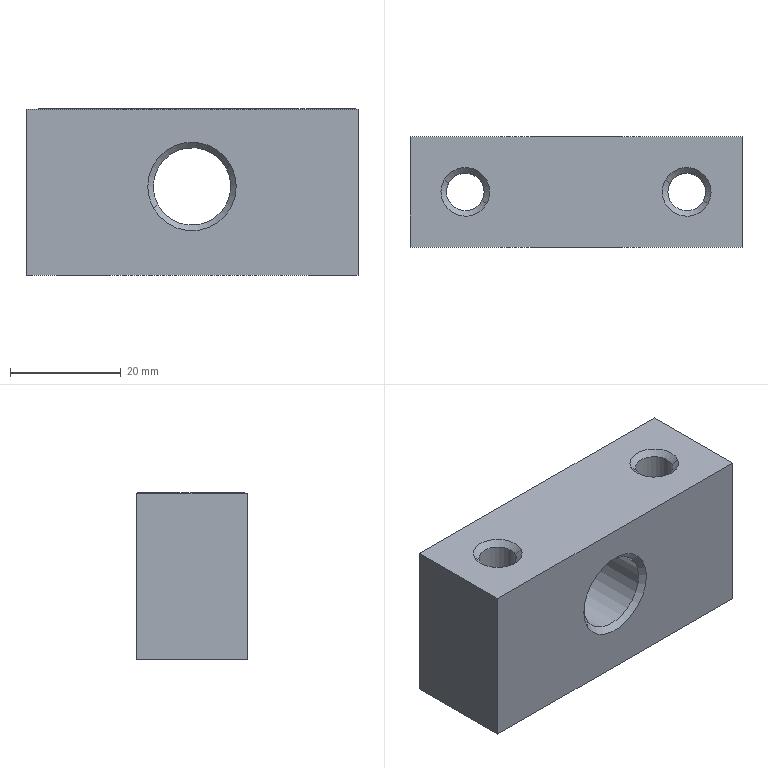Part | STEP file | 20303 | 1 solid | 24 faces | box 60 x 20 x 30 mm | volume 30649 mm3 | cone 12 | plane 6 | cylinder 6 | commonest cylinder face diameters 6.8 x4 14 x2
STEP:
#1=CARTESIAN_POINT('',(30.,-10.,0.));
#2=VERTEX_POINT('',#1);
#3=CARTESIAN_POINT('',(30.,-10.,30.));
#4=VERTEX_POINT('',#3);
#5=CARTESIAN_POINT('',(30.,-10.,15.));
#6=DIRECTION('',(0.,0.,1.));
#7=VECTOR('',#6,1.);
#8=LINE('',#5,#7);
#9=EDGE_CURVE('',#2,#4,#8,.T.);
#10=ORIENTED_EDGE('',*,*,#9,.F.);
#11=CARTESIAN_POINT('',(30.,10.,0.));
#12=VERTEX_POINT('',#11);
#13=CARTESIAN_POINT('',(30.,0.,0.));
#14=DIRECTION('',(0.,-1.,0.));
#15=VECTOR('',#14,1.);
#16=LINE('',#13,#15);
#17=EDGE_CURVE('',#2,#12,#16,.F.);
#18=ORIENTED_EDGE('',*,*,#17,.T.);
#19=CARTESIAN_POINT('',(30.,10.,30.));
#20=VERTEX_POINT('',#19);
#21=CARTESIAN_POINT('',(30.,10.,15.));
#22=DIRECTION('',(0.,0.,1.));
#23=VECTOR('',#22,1.);
#24=LINE('',#21,#23);
#25=EDGE_CURVE('',#12,#20,#24,.T.);
#26=ORIENTED_EDGE('',*,*,#25,.T.);
#27=CARTESIAN_POINT('',(30.,0.,30.));
#28=DIRECTION('',(0.,-1.,0.));
#29=VECTOR('',#28,1.);
#30=LINE('',#27,#29);
#31=EDGE_CURVE('',#4,#20,#30,.F.);
#32=ORIENTED_EDGE('',*,*,#31,.F.);
#33=EDGE_LOOP('',(#10,#18,#26,#32));
#34=FACE_OUTER_BOUND('',#33,.T.);
#35=CARTESIAN_POINT('',(30.,10.,0.));
#36=DIRECTION('',(-1.,0.,0.));
#37=DIRECTION('',(0.,-1.,0.));
#38=AXIS2_PLACEMENT_3D('',#35,#36,#37);
#39=PLANE('',#38);
#40=ADVANCED_FACE('',(#34),#39,.F.);
#41=CARTESIAN_POINT('',(-30.,10.,0.));
#42=VERTEX_POINT('',#41);
#43=CARTESIAN_POINT('',(-30.,10.,30.));
#44=VERTEX_POINT('',#43);
#45=CARTESIAN_POINT('',(-30.,10.,15.));
#46=DIRECTION('',(0.,0.,1.));
#47=VECTOR('',#46,1.);
#48=LINE('',#45,#47);
#49=EDGE_CURVE('',#42,#44,#48,.T.);
#50=ORIENTED_EDGE('',*,*,#49,.F.);
#51=CARTESIAN_POINT('',(-30.,-10.,0.));
#52=VERTEX_POINT('',#51);
#53=CARTESIAN_POINT('',(-30.,0.,0.));
#54=DIRECTION('',(0.,1.,0.));
#55=VECTOR('',#54,1.);
#56=LINE('',#53,#55);
#57=EDGE_CURVE('',#42,#52,#56,.F.);
#58=ORIENTED_EDGE('',*,*,#57,.T.);
#59=CARTESIAN_POINT('',(-30.,-10.,30.));
#60=VERTEX_POINT('',#59);
#61=CARTESIAN_POINT('',(-30.,-10.,15.));
#62=DIRECTION('',(0.,0.,1.));
#63=VECTOR('',#62,1.);
#64=LINE('',#61,#63);
#65=EDGE_CURVE('',#52,#60,#64,.T.);
#66=ORIENTED_EDGE('',*,*,#65,.T.);
#67=CARTESIAN_POINT('',(-30.,0.,30.));
#68=DIRECTION('',(0.,1.,0.));
#69=VECTOR('',#68,1.);
#70=LINE('',#67,#69);
#71=EDGE_CURVE('',#44,#60,#70,.F.);
#72=ORIENTED_EDGE('',*,*,#71,.F.);
#73=EDGE_LOOP('',(#50,#58,#66,#72));
#74=FACE_OUTER_BOUND('',#73,.T.);
#75=CARTESIAN_POINT('',(-30.,-10.,0.));
#76=DIRECTION('',(1.,0.,0.));
#77=DIRECTION('',(0.,1.,0.));
#78=AXIS2_PLACEMENT_3D('',#75,#76,#77);
#79=PLANE('',#78);
#80=ADVANCED_FACE('',(#74),#79,.F.);
#81=CARTESIAN_POINT('',(17.016,1.63,1.));
#82=VERTEX_POINT('',#81);
#83=CARTESIAN_POINT('',(16.139,2.109,0.));
#84=VERTEX_POINT('',#83);
#85=CARTESIAN_POINT('',(16.577,1.87,0.5));
#86=DIRECTION('',(-0.6205,0.339,-0.7071));
#87=VECTOR('',#86,1.);
#88=LINE('',#85,#87);
#89=EDGE_CURVE('',#82,#84,#88,.T.);
#90=ORIENTED_EDGE('',*,*,#89,.T.);
#91=CARTESIAN_POINT('',(23.861,-2.109,0.));
#92=VERTEX_POINT('',#91);
#93=CARTESIAN_POINT('',(20.,0.,0.));
#94=DIRECTION('',(0.,0.,1.));
#95=AXIS2_PLACEMENT_3D('',#93,#94,$);
#96=CIRCLE('',#95,4.4);
#97=EDGE_CURVE('',#84,#92,#96,.F.);
#98=ORIENTED_EDGE('',*,*,#97,.T.);
#99=CARTESIAN_POINT('',(22.984,-1.63,1.));
#100=VERTEX_POINT('',#99);
#101=CARTESIAN_POINT('',(23.423,-1.87,0.5));
#102=DIRECTION('',(0.6205,-0.339,-0.7071));
#103=VECTOR('',#102,1.);
#104=LINE('',#101,#103);
#105=EDGE_CURVE('',#100,#92,#104,.T.);
#106=ORIENTED_EDGE('',*,*,#105,.F.);
#107=CARTESIAN_POINT('',(20.,0.,1.));
#108=DIRECTION('',(0.,0.,1.));
#109=AXIS2_PLACEMENT_3D('',#107,#108,$);
#110=CIRCLE('',#109,3.4);
#111=EDGE_CURVE('',#82,#100,#110,.F.);
#112=ORIENTED_EDGE('',*,*,#111,.F.);
#113=EDGE_LOOP('',(#90,#98,#106,#112));
#114=FACE_OUTER_BOUND('',#113,.T.);
#115=CARTESIAN_POINT('',(20.,0.,4.4));
#116=DIRECTION('',(0.,0.,-1.));
#117=DIRECTION('',(0.8776,-0.4794,0.));
#118=AXIS2_PLACEMENT_3D('',#115,#116,#117);
#119=CONICAL_SURFACE('',#118,0.,0.7854);
#120=ADVANCED_FACE('',(#114),#119,.F.);
#121=ORIENTED_EDGE('',*,*,#105,.T.);
#122=CARTESIAN_POINT('',(20.,0.,0.));
#123=DIRECTION('',(0.,0.,1.));
#124=AXIS2_PLACEMENT_3D('',#122,#123,$);
#125=CIRCLE('',#124,4.4);
#126=EDGE_CURVE('',#92,#84,#125,.F.);
#127=ORIENTED_EDGE('',*,*,#126,.T.);
#128=ORIENTED_EDGE('',*,*,#89,.F.);
#129=CARTESIAN_POINT('',(20.,0.,1.));
#130=DIRECTION('',(0.,0.,1.));
#131=AXIS2_PLACEMENT_3D('',#129,#130,$);
#132=CIRCLE('',#131,3.4);
#133=EDGE_CURVE('',#100,#82,#132,.F.);
#134=ORIENTED_EDGE('',*,*,#133,.F.);
#135=EDGE_LOOP('',(#121,#127,#128,#134));
#136=FACE_OUTER_BOUND('',#135,.T.);
#137=CARTESIAN_POINT('',(20.,0.,4.4));
#138=DIRECTION('',(0.,0.,-1.));
#139=DIRECTION('',(-0.5949,0.8038,0.));
#140=AXIS2_PLACEMENT_3D('',#137,#138,#139);
#141=CONICAL_SURFACE('',#140,0.,0.7854);
#142=ADVANCED_FACE('',(#136),#141,.F.);
#143=CARTESIAN_POINT('',(22.984,-1.63,29.));
#144=VERTEX_POINT('',#143);
#145=CARTESIAN_POINT('',(17.016,1.63,29.));
#146=VERTEX_POINT('',#145);
#147=CARTESIAN_POINT('',(20.,0.,29.));
#148=DIRECTION('',(0.,0.,-1.));
#149=AXIS2_PLACEMENT_3D('',#147,#148,$);
#150=CIRCLE('',#149,3.4);
#151=EDGE_CURVE('',#144,#146,#150,.F.);
#152=ORIENTED_EDGE('',*,*,#151,.T.);
#153=CARTESIAN_POINT('',(17.016,1.63,15.155));
#154=DIRECTION('',(0.,0.,-1.));
#155=VECTOR('',#154,1.);
#156=LINE('',#153,#155);
#157=EDGE_CURVE('',#82,#146,#156,.F.);
#158=ORIENTED_EDGE('',*,*,#157,.F.);
#159=ORIENTED_EDGE('',*,*,#111,.T.);
#160=CARTESIAN_POINT('',(22.984,-1.63,15.155));
#161=DIRECTION('',(0.,0.,-1.));
#162=VECTOR('',#161,1.);
#163=LINE('',#160,#162);
#164=EDGE_CURVE('',#100,#144,#163,.F.);
#165=ORIENTED_EDGE('',*,*,#164,.T.);
#166=EDGE_LOOP('',(#152,#158,#159,#165));
#167=FACE_OUTER_BOUND('',#166,.T.);
#168=CARTESIAN_POINT('',(20.,0.,29.9));
#169=DIRECTION('',(0.,0.,-1.));
#170=DIRECTION('',(0.8776,-0.4794,0.));
#171=AXIS2_PLACEMENT_3D('',#168,#169,#170);
#172=CYLINDRICAL_SURFACE('',#171,3.4);
#173=ADVANCED_FACE('',(#167),#172,.F.);
#174=CARTESIAN_POINT('',(20.,0.,29.));
#175=DIRECTION('',(0.,0.,-1.));
#176=AXIS2_PLACEMENT_3D('',#174,#175,$);
#177=CIRCLE('',#176,3.4);
#178=EDGE_CURVE('',#146,#144,#177,.F.);
#179=ORIENTED_EDGE('',*,*,#178,.T.);
#180=ORIENTED_EDGE('',*,*,#164,.F.);
#181=ORIENTED_EDGE('',*,*,#133,.T.);
#182=ORIENTED_EDGE('',*,*,#157,.T.);
#183=EDGE_LOOP('',(#179,#180,#181,#182));
#184=FACE_OUTER_BOUND('',#183,.T.);
#185=ADVANCED_FACE('',(#184),#172,.F.);
#186=CARTESIAN_POINT('',(23.861,-2.109,30.));
#187=VERTEX_POINT('',#186);
#188=CARTESIAN_POINT('',(23.423,-1.87,29.5));
#189=DIRECTION('',(0.6205,-0.339,0.7071));
#190=VECTOR('',#189,1.);
#191=LINE('',#188,#190);
#192=EDGE_CURVE('',#144,#187,#191,.T.);
#193=ORIENTED_EDGE('',*,*,#192,.T.);
#194=CARTESIAN_POINT('',(16.139,2.109,30.));
#195=VERTEX_POINT('',#194);
#196=CARTESIAN_POINT('',(20.,0.,30.));
#197=DIRECTION('',(0.,0.,1.));
#198=AXIS2_PLACEMENT_3D('',#196,#197,$);
#199=CIRCLE('',#198,4.4);
#200=EDGE_CURVE('',#187,#195,#199,.T.);
#201=ORIENTED_EDGE('',*,*,#200,.T.);
#202=CARTESIAN_POINT('',(16.577,1.87,29.5));
#203=DIRECTION('',(-0.6205,0.339,0.7071));
#204=VECTOR('',#203,1.);
#205=LINE('',#202,#204);
#206=EDGE_CURVE('',#146,#195,#205,.T.);
#207=ORIENTED_EDGE('',*,*,#206,.F.);
#208=ORIENTED_EDGE('',*,*,#151,.F.);
#209=EDGE_LOOP('',(#193,#201,#207,#208));
#210=FACE_OUTER_BOUND('',#209,.T.);
#211=CARTESIAN_POINT('',(20.,0.,25.6));
#212=DIRECTION('',(0.,0.,1.));
#213=DIRECTION('',(0.8776,-0.4794,0.));
#214=AXIS2_PLACEMENT_3D('',#211,#212,#213);
#215=CONICAL_SURFACE('',#214,0.,0.7854);
#216=ADVANCED_FACE('',(#210),#215,.F.);
#217=ORIENTED_EDGE('',*,*,#206,.T.);
#218=CARTESIAN_POINT('',(20.,0.,30.));
#219=DIRECTION('',(0.,0.,1.));
#220=AXIS2_PLACEMENT_3D('',#218,#219,$);
#221=CIRCLE('',#220,4.4);
#222=EDGE_CURVE('',#195,#187,#221,.T.);
#223=ORIENTED_EDGE('',*,*,#222,.T.);
#224=ORIENTED_EDGE('',*,*,#192,.F.);
#225=ORIENTED_EDGE('',*,*,#178,.F.);
#226=EDGE_LOOP('',(#217,#223,#224,#225));
#227=FACE_OUTER_BOUND('',#226,.T.);
#228=CARTESIAN_POINT('',(20.,0.,25.6));
#229=DIRECTION('',(0.,0.,1.));
#230=DIRECTION('',(-0.5851,0.811,0.));
#231=AXIS2_PLACEMENT_3D('',#228,#229,#230);
#232=CONICAL_SURFACE('',#231,0.,0.7854);
#233=ADVANCED_FACE('',(#227),#232,.F.);
#234=ORIENTED_EDGE('',*,*,#17,.F.);
#235=CARTESIAN_POINT('',(0.,-10.,0.));
#236=DIRECTION('',(-1.,0.,0.));
#237=VECTOR('',#236,1.);
#238=LINE('',#235,#237);
#239=EDGE_CURVE('',#52,#2,#238,.F.);
#240=ORIENTED_EDGE('',*,*,#239,.F.);
#241=ORIENTED_EDGE('',*,*,#57,.F.);
#242=CARTESIAN_POINT('',(0.,10.,0.));
#243=DIRECTION('',(1.,0.,0.));
#244=VECTOR('',#243,1.);
#245=LINE('',#242,#244);
#246=EDGE_CURVE('',#12,#42,#245,.F.);
#247=ORIENTED_EDGE('',*,*,#246,.F.);
#248=EDGE_LOOP('',(#234,#240,#241,#247));
#249=FACE_OUTER_BOUND('',#248,.T.);
#250=CARTESIAN_POINT('',(-23.861,2.109,0.));
#251=VERTEX_POINT('',#250);
#252=CARTESIAN_POINT('',(-16.139,-2.109,0.));
#253=VERTEX_POINT('',#252);
#254=CARTESIAN_POINT('',(-20.,0.,0.));
#255=DIRECTION('',(0.,0.,1.));
#256=AXIS2_PLACEMENT_3D('',#254,#255,$);
#257=CIRCLE('',#256,4.4);
#258=EDGE_CURVE('',#251,#253,#257,.F.);
#259=ORIENTED_EDGE('',*,*,#258,.F.);
#260=CARTESIAN_POINT('',(-20.,0.,0.));
#261=DIRECTION('',(0.,0.,1.));
#262=AXIS2_PLACEMENT_3D('',#260,#261,$);
#263=CIRCLE('',#262,4.4);
#264=EDGE_CURVE('',#253,#251,#263,.F.);
#265=ORIENTED_EDGE('',*,*,#264,.F.);
#266=EDGE_LOOP('',(#259,#265));
#267=FACE_BOUND('',#266,.T.);
#268=ORIENTED_EDGE('',*,*,#97,.F.);
#269=ORIENTED_EDGE('',*,*,#126,.F.);
#270=EDGE_LOOP('',(#268,#269));
#271=FACE_BOUND('',#270,.T.);
#272=CARTESIAN_POINT('',(0.,0.,0.));
#273=DIRECTION('',(0.,0.,1.));
#274=DIRECTION('',(1.,0.,0.));
#275=AXIS2_PLACEMENT_3D('',#272,#273,#274);
#276=PLANE('',#275);
#277=ADVANCED_FACE('',(#249,#267,#271),#276,.F.);
#278=CARTESIAN_POINT('',(-22.984,1.63,1.));
#279=VERTEX_POINT('',#278);
#280=CARTESIAN_POINT('',(-23.423,1.87,0.5));
#281=DIRECTION('',(-0.6205,0.339,-0.7071));
#282=VECTOR('',#281,1.);
#283=LINE('',#280,#282);
#284=EDGE_CURVE('',#279,#251,#283,.T.);
#285=ORIENTED_EDGE('',*,*,#284,.T.);
#286=ORIENTED_EDGE('',*,*,#258,.T.);
#287=CARTESIAN_POINT('',(-17.016,-1.63,1.));
#288=VERTEX_POINT('',#287);
#289=CARTESIAN_POINT('',(-16.577,-1.87,0.5));
#290=DIRECTION('',(0.6205,-0.339,-0.7071));
#291=VECTOR('',#290,1.);
#292=LINE('',#289,#291);
#293=EDGE_CURVE('',#288,#253,#292,.T.);
#294=ORIENTED_EDGE('',*,*,#293,.F.);
#295=CARTESIAN_POINT('',(-20.,0.,1.));
#296=DIRECTION('',(0.,0.,1.));
#297=AXIS2_PLACEMENT_3D('',#295,#296,$);
#298=CIRCLE('',#297,3.4);
#299=EDGE_CURVE('',#279,#288,#298,.F.);
#300=ORIENTED_EDGE('',*,*,#299,.F.);
#301=EDGE_LOOP('',(#285,#286,#294,#300));
#302=FACE_OUTER_BOUND('',#301,.T.);
#303=CARTESIAN_POINT('',(-20.,0.,4.4));
#304=DIRECTION('',(0.,0.,-1.));
#305=DIRECTION('',(0.8776,-0.4794,0.));
#306=AXIS2_PLACEMENT_3D('',#303,#304,#305);
#307=CONICAL_SURFACE('',#306,0.,0.7854);
#308=ADVANCED_FACE('',(#302),#307,.F.);
#309=ORIENTED_EDGE('',*,*,#293,.T.);
#310=ORIENTED_EDGE('',*,*,#264,.T.);
#311=ORIENTED_EDGE('',*,*,#284,.F.);
#312=CARTESIAN_POINT('',(-20.,0.,1.));
#313=DIRECTION('',(0.,0.,1.));
#314=AXIS2_PLACEMENT_3D('',#312,#313,$);
#315=CIRCLE('',#314,3.4);
#316=EDGE_CURVE('',#288,#279,#315,.F.);
#317=ORIENTED_EDGE('',*,*,#316,.F.);
#318=EDGE_LOOP('',(#309,#310,#311,#317));
#319=FACE_OUTER_BOUND('',#318,.T.);
#320=CARTESIAN_POINT('',(-20.,0.,4.4));
#321=DIRECTION('',(0.,0.,-1.));
#322=DIRECTION('',(-0.5949,0.8038,0.));
#323=AXIS2_PLACEMENT_3D('',#320,#321,#322);
#324=CONICAL_SURFACE('',#323,0.,0.7854);
#325=ADVANCED_FACE('',(#319),#324,.F.);
#326=CARTESIAN_POINT('',(0.,10.,30.));
#327=DIRECTION('',(1.,0.,0.));
#328=VECTOR('',#327,1.);
#329=LINE('',#326,#328);
#330=EDGE_CURVE('',#20,#44,#329,.F.);
#331=ORIENTED_EDGE('',*,*,#330,.T.);
#332=ORIENTED_EDGE('',*,*,#71,.T.);
#333=CARTESIAN_POINT('',(0.,-10.,30.));
#334=DIRECTION('',(-1.,0.,0.));
#335=VECTOR('',#334,1.);
#336=LINE('',#333,#335);
#337=EDGE_CURVE('',#60,#4,#336,.F.);
#338=ORIENTED_EDGE('',*,*,#337,.T.);
#339=ORIENTED_EDGE('',*,*,#31,.T.);
#340=EDGE_LOOP('',(#331,#332,#338,#339));
#341=FACE_OUTER_BOUND('',#340,.T.);
#342=CARTESIAN_POINT('',(-23.861,2.109,30.));
#343=VERTEX_POINT('',#342);
#344=CARTESIAN_POINT('',(-16.139,-2.109,30.));
#345=VERTEX_POINT('',#344);
#346=CARTESIAN_POINT('',(-20.,0.,30.));
#347=DIRECTION('',(0.,0.,1.));
#348=AXIS2_PLACEMENT_3D('',#346,#347,$);
#349=CIRCLE('',#348,4.4);
#350=EDGE_CURVE('',#343,#345,#349,.T.);
#351=ORIENTED_EDGE('',*,*,#350,.F.);
#352=CARTESIAN_POINT('',(-20.,0.,30.));
#353=DIRECTION('',(0.,0.,1.));
#354=AXIS2_PLACEMENT_3D('',#352,#353,$);
#355=CIRCLE('',#354,4.4);
#356=EDGE_CURVE('',#345,#343,#355,.T.);
#357=ORIENTED_EDGE('',*,*,#356,.F.);
#358=EDGE_LOOP('',(#351,#357));
#359=FACE_BOUND('',#358,.T.);
#360=ORIENTED_EDGE('',*,*,#222,.F.);
#361=ORIENTED_EDGE('',*,*,#200,.F.);
#362=EDGE_LOOP('',(#360,#361));
#363=FACE_BOUND('',#362,.T.);
#364=CARTESIAN_POINT('',(0.,0.,30.));
#365=DIRECTION('',(0.,0.,1.));
#366=DIRECTION('',(1.,0.,0.));
#367=AXIS2_PLACEMENT_3D('',#364,#365,#366);
#368=PLANE('',#367);
#369=ADVANCED_FACE('',(#341,#359,#363),#368,.T.);
#370=CARTESIAN_POINT('',(-17.016,-1.63,29.));
#371=VERTEX_POINT('',#370);
#372=CARTESIAN_POINT('',(-22.984,1.63,29.));
#373=VERTEX_POINT('',#372);
#374=CARTESIAN_POINT('',(-20.,0.,29.));
#375=DIRECTION('',(0.,0.,-1.));
#376=AXIS2_PLACEMENT_3D('',#374,#375,$);
#377=CIRCLE('',#376,3.4);
#378=EDGE_CURVE('',#371,#373,#377,.F.);
#379=ORIENTED_EDGE('',*,*,#378,.T.);
#380=CARTESIAN_POINT('',(-22.984,1.63,15.155));
#381=DIRECTION('',(0.,0.,-1.));
#382=VECTOR('',#381,1.);
#383=LINE('',#380,#382);
#384=EDGE_CURVE('',#279,#373,#383,.F.);
#385=ORIENTED_EDGE('',*,*,#384,.F.);
#386=ORIENTED_EDGE('',*,*,#299,.T.);
#387=CARTESIAN_POINT('',(-17.016,-1.63,15.155));
#388=DIRECTION('',(0.,0.,-1.));
#389=VECTOR('',#388,1.);
#390=LINE('',#387,#389);
#391=EDGE_CURVE('',#288,#371,#390,.F.);
#392=ORIENTED_EDGE('',*,*,#391,.T.);
#393=EDGE_LOOP('',(#379,#385,#386,#392));
#394=FACE_OUTER_BOUND('',#393,.T.);
#395=CARTESIAN_POINT('',(-20.,0.,29.9));
#396=DIRECTION('',(0.,0.,-1.));
#397=DIRECTION('',(0.8776,-0.4794,0.));
#398=AXIS2_PLACEMENT_3D('',#395,#396,#397);
#399=CYLINDRICAL_SURFACE('',#398,3.4);
#400=ADVANCED_FACE('',(#394),#399,.F.);
#401=CARTESIAN_POINT('',(-20.,0.,29.));
#402=DIRECTION('',(0.,0.,-1.));
#403=AXIS2_PLACEMENT_3D('',#401,#402,$);
#404=CIRCLE('',#403,3.4);
#405=EDGE_CURVE('',#373,#371,#404,.F.);
#406=ORIENTED_EDGE('',*,*,#405,.T.);
#407=ORIENTED_EDGE('',*,*,#391,.F.);
#408=ORIENTED_EDGE('',*,*,#316,.T.);
#409=ORIENTED_EDGE('',*,*,#384,.T.);
#410=EDGE_LOOP('',(#406,#407,#408,#409));
#411=FACE_OUTER_BOUND('',#410,.T.);
#412=ADVANCED_FACE('',(#411),#399,.F.);
#413=CARTESIAN_POINT('',(-16.577,-1.87,29.5));
#414=DIRECTION('',(0.6205,-0.339,0.7071));
#415=VECTOR('',#414,1.);
#416=LINE('',#413,#415);
#417=EDGE_CURVE('',#371,#345,#416,.T.);
#418=ORIENTED_EDGE('',*,*,#417,.T.);
#419=ORIENTED_EDGE('',*,*,#356,.T.);
#420=CARTESIAN_POINT('',(-23.423,1.87,29.5));
#421=DIRECTION('',(-0.6205,0.339,0.7071));
#422=VECTOR('',#421,1.);
#423=LINE('',#420,#422);
#424=EDGE_CURVE('',#373,#343,#423,.T.);
#425=ORIENTED_EDGE('',*,*,#424,.F.);
#426=ORIENTED_EDGE('',*,*,#378,.F.);
#427=EDGE_LOOP('',(#418,#419,#425,#426));
#428=FACE_OUTER_BOUND('',#427,.T.);
#429=CARTESIAN_POINT('',(-20.,0.,25.6));
#430=DIRECTION('',(0.,0.,1.));
#431=DIRECTION('',(0.8776,-0.4794,0.));
#432=AXIS2_PLACEMENT_3D('',#429,#430,#431);
#433=CONICAL_SURFACE('',#432,0.,0.7854);
#434=ADVANCED_FACE('',(#428),#433,.F.);
#435=ORIENTED_EDGE('',*,*,#424,.T.);
#436=ORIENTED_EDGE('',*,*,#350,.T.);
#437=ORIENTED_EDGE('',*,*,#417,.F.);
#438=ORIENTED_EDGE('',*,*,#405,.F.);
#439=EDGE_LOOP('',(#435,#436,#437,#438));
#440=FACE_OUTER_BOUND('',#439,.T.);
#441=CARTESIAN_POINT('',(-20.,0.,25.6));
#442=DIRECTION('',(0.,0.,1.));
#443=DIRECTION('',(-0.5851,0.811,0.));
#444=AXIS2_PLACEMENT_3D('',#441,#442,#443);
#445=CONICAL_SURFACE('',#444,0.,0.7854);
#446=ADVANCED_FACE('',(#440),#445,.F.);
#447=ORIENTED_EDGE('',*,*,#65,.F.);
#448=ORIENTED_EDGE('',*,*,#239,.T.);
#449=ORIENTED_EDGE('',*,*,#9,.T.);
#450=ORIENTED_EDGE('',*,*,#337,.F.);
#451=EDGE_LOOP('',(#447,#448,#449,#450));
#452=FACE_OUTER_BOUND('',#451,.T.);
#453=CARTESIAN_POINT('',(7.021,-10.,19.835));
#454=VERTEX_POINT('',#453);
#455=CARTESIAN_POINT('',(-7.021,-10.,12.165));
#456=VERTEX_POINT('',#455);
#457=CARTESIAN_POINT('',(0.,-10.,16.));
#458=DIRECTION('',(0.,1.,0.));
#459=AXIS2_PLACEMENT_3D('',#457,#458,$);
#460=CIRCLE('',#459,8.);
#461=EDGE_CURVE('',#454,#456,#460,.F.);
#462=ORIENTED_EDGE('',*,*,#461,.F.);
#463=CARTESIAN_POINT('',(0.,-10.,16.));
#464=DIRECTION('',(0.,1.,0.));
#465=AXIS2_PLACEMENT_3D('',#463,#464,$);
#466=CIRCLE('',#465,8.);
#467=EDGE_CURVE('',#456,#454,#466,.F.);
#468=ORIENTED_EDGE('',*,*,#467,.F.);
#469=EDGE_LOOP('',(#462,#468));
#470=FACE_BOUND('',#469,.T.);
#471=CARTESIAN_POINT('',(30.,-10.,0.));
#472=DIRECTION('',(0.,1.,0.));
#473=DIRECTION('',(-1.,0.,0.));
#474=AXIS2_PLACEMENT_3D('',#471,#472,#473);
#475=PLANE('',#474);
#476=ADVANCED_FACE('',(#452,#470),#475,.F.);
#477=CARTESIAN_POINT('',(6.143,-9.,19.356));
#478=VERTEX_POINT('',#477);
#479=CARTESIAN_POINT('',(6.582,-9.5,19.596));
#480=DIRECTION('',(0.6205,-0.7071,0.339));
#481=VECTOR('',#480,1.);
#482=LINE('',#479,#481);
#483=EDGE_CURVE('',#478,#454,#482,.T.);
#484=ORIENTED_EDGE('',*,*,#483,.T.);
#485=ORIENTED_EDGE('',*,*,#461,.T.);
#486=CARTESIAN_POINT('',(-6.143,-9.,12.644));
#487=VERTEX_POINT('',#486);
#488=CARTESIAN_POINT('',(-6.582,-9.5,12.404));
#489=DIRECTION('',(-0.6205,-0.7071,-0.339));
#490=VECTOR('',#489,1.);
#491=LINE('',#488,#490);
#492=EDGE_CURVE('',#487,#456,#491,.T.);
#493=ORIENTED_EDGE('',*,*,#492,.F.);
#494=CARTESIAN_POINT('',(0.,-9.,16.));
#495=DIRECTION('',(0.,1.,0.));
#496=AXIS2_PLACEMENT_3D('',#494,#495,$);
#497=CIRCLE('',#496,7.);
#498=EDGE_CURVE('',#478,#487,#497,.F.);
#499=ORIENTED_EDGE('',*,*,#498,.F.);
#500=EDGE_LOOP('',(#484,#485,#493,#499));
#501=FACE_OUTER_BOUND('',#500,.T.);
#502=CARTESIAN_POINT('',(0.,-2.,16.));
#503=DIRECTION('',(0.,-1.,0.));
#504=DIRECTION('',(-0.7395,0.,-0.6732));
#505=AXIS2_PLACEMENT_3D('',#502,#503,#504);
#506=CONICAL_SURFACE('',#505,0.,0.7854);
#507=ADVANCED_FACE('',(#501),#506,.F.);
#508=ORIENTED_EDGE('',*,*,#492,.T.);
#509=ORIENTED_EDGE('',*,*,#467,.T.);
#510=ORIENTED_EDGE('',*,*,#483,.F.);
#511=CARTESIAN_POINT('',(0.,-9.,16.));
#512=DIRECTION('',(0.,1.,0.));
#513=AXIS2_PLACEMENT_3D('',#511,#512,$);
#514=CIRCLE('',#513,7.);
#515=EDGE_CURVE('',#487,#478,#514,.F.);
#516=ORIENTED_EDGE('',*,*,#515,.F.);
#517=EDGE_LOOP('',(#508,#509,#510,#516));
#518=FACE_OUTER_BOUND('',#517,.T.);
#519=CARTESIAN_POINT('',(0.,-2.,16.));
#520=DIRECTION('',(0.,-1.,0.));
#521=DIRECTION('',(0.8776,0.,0.4794));
#522=AXIS2_PLACEMENT_3D('',#519,#520,#521);
#523=CONICAL_SURFACE('',#522,0.,0.7854);
#524=ADVANCED_FACE('',(#518),#523,.F.);
#525=ORIENTED_EDGE('',*,*,#25,.F.);
#526=ORIENTED_EDGE('',*,*,#246,.T.);
#527=ORIENTED_EDGE('',*,*,#49,.T.);
#528=ORIENTED_EDGE('',*,*,#330,.F.);
#529=EDGE_LOOP('',(#525,#526,#527,#528));
#530=FACE_OUTER_BOUND('',#529,.T.);
#531=CARTESIAN_POINT('',(7.021,10.,19.835));
#532=VERTEX_POINT('',#531);
#533=CARTESIAN_POINT('',(-7.021,10.,12.165));
#534=VERTEX_POINT('',#533);
#535=CARTESIAN_POINT('',(0.,10.,16.));
#536=DIRECTION('',(0.,-1.,0.));
#537=AXIS2_PLACEMENT_3D('',#535,#536,$);
#538=CIRCLE('',#537,8.);
#539=EDGE_CURVE('',#532,#534,#538,.T.);
#540=ORIENTED_EDGE('',*,*,#539,.T.);
#541=CARTESIAN_POINT('',(0.,10.,16.));
#542=DIRECTION('',(0.,-1.,0.));
#543=AXIS2_PLACEMENT_3D('',#541,#542,$);
#544=CIRCLE('',#543,8.);
#545=EDGE_CURVE('',#534,#532,#544,.T.);
#546=ORIENTED_EDGE('',*,*,#545,.T.);
#547=EDGE_LOOP('',(#540,#546));
#548=FACE_BOUND('',#547,.T.);
#549=CARTESIAN_POINT('',(-30.,10.,0.));
#550=DIRECTION('',(0.,-1.,0.));
#551=DIRECTION('',(1.,0.,0.));
#552=AXIS2_PLACEMENT_3D('',#549,#550,#551);
#553=PLANE('',#552);
#554=ADVANCED_FACE('',(#530,#548),#553,.F.);
#555=CARTESIAN_POINT('',(6.143,9.,19.356));
#556=VERTEX_POINT('',#555);
#557=CARTESIAN_POINT('',(-6.143,9.,12.644));
#558=VERTEX_POINT('',#557);
#559=CARTESIAN_POINT('',(0.,9.,16.));
#560=DIRECTION('',(0.,-1.,0.));
#561=AXIS2_PLACEMENT_3D('',#559,#560,$);
#562=CIRCLE('',#561,7.);
#563=EDGE_CURVE('',#556,#558,#562,.T.);
#564=ORIENTED_EDGE('',*,*,#563,.F.);
#565=CARTESIAN_POINT('',(6.143,0.155,19.356));
#566=DIRECTION('',(0.,-1.,0.));
#567=VECTOR('',#566,1.);
#568=LINE('',#565,#567);
#569=EDGE_CURVE('',#478,#556,#568,.F.);
#570=ORIENTED_EDGE('',*,*,#569,.F.);
#571=ORIENTED_EDGE('',*,*,#498,.T.);
#572=CARTESIAN_POINT('',(-6.143,0.155,12.644));
#573=DIRECTION('',(0.,-1.,0.));
#574=VECTOR('',#573,1.);
#575=LINE('',#572,#574);
#576=EDGE_CURVE('',#487,#558,#575,.F.);
#577=ORIENTED_EDGE('',*,*,#576,.T.);
#578=EDGE_LOOP('',(#564,#570,#571,#577));
#579=FACE_OUTER_BOUND('',#578,.T.);
#580=CARTESIAN_POINT('',(0.,9.9,16.));
#581=DIRECTION('',(0.,-1.,0.));
#582=DIRECTION('',(0.8776,0.,0.4794));
#583=AXIS2_PLACEMENT_3D('',#580,#581,#582);
#584=CYLINDRICAL_SURFACE('',#583,7.);
#585=ADVANCED_FACE('',(#579),#584,.F.);
#586=CARTESIAN_POINT('',(0.,9.,16.));
#587=DIRECTION('',(0.,-1.,0.));
#588=AXIS2_PLACEMENT_3D('',#586,#587,$);
#589=CIRCLE('',#588,7.);
#590=EDGE_CURVE('',#558,#556,#589,.T.);
#591=ORIENTED_EDGE('',*,*,#590,.F.);
#592=ORIENTED_EDGE('',*,*,#576,.F.);
#593=ORIENTED_EDGE('',*,*,#515,.T.);
#594=ORIENTED_EDGE('',*,*,#569,.T.);
#595=EDGE_LOOP('',(#591,#592,#593,#594));
#596=FACE_OUTER_BOUND('',#595,.T.);
#597=ADVANCED_FACE('',(#596),#584,.F.);
#598=CARTESIAN_POINT('',(6.582,9.5,19.596));
#599=DIRECTION('',(0.6205,0.7071,0.339));
#600=VECTOR('',#599,1.);
#601=LINE('',#598,#600);
#602=EDGE_CURVE('',#532,#556,#601,.F.);
#603=ORIENTED_EDGE('',*,*,#602,.T.);
#604=ORIENTED_EDGE('',*,*,#563,.T.);
#605=CARTESIAN_POINT('',(-6.582,9.5,12.404));
#606=DIRECTION('',(-0.6205,0.7071,-0.339));
#607=VECTOR('',#606,1.);
#608=LINE('',#605,#607);
#609=EDGE_CURVE('',#534,#558,#608,.F.);
#610=ORIENTED_EDGE('',*,*,#609,.F.);
#611=ORIENTED_EDGE('',*,*,#539,.F.);
#612=EDGE_LOOP('',(#603,#604,#610,#611));
#613=FACE_OUTER_BOUND('',#612,.T.);
#614=CARTESIAN_POINT('',(0.,2.,16.));
#615=DIRECTION('',(0.,1.,0.));
#616=DIRECTION('',(0.8776,0.,0.4794));
#617=AXIS2_PLACEMENT_3D('',#614,#615,#616);
#618=CONICAL_SURFACE('',#617,0.,0.7854);
#619=ADVANCED_FACE('',(#613),#618,.F.);
#620=ORIENTED_EDGE('',*,*,#609,.T.);
#621=ORIENTED_EDGE('',*,*,#590,.T.);
#622=ORIENTED_EDGE('',*,*,#602,.F.);
#623=ORIENTED_EDGE('',*,*,#545,.F.);
#624=EDGE_LOOP('',(#620,#621,#622,#623));
#625=FACE_OUTER_BOUND('',#624,.T.);
#626=CARTESIAN_POINT('',(0.,2.,16.));
#627=DIRECTION('',(0.,1.,0.));
#628=DIRECTION('',(-1.,0.,-0.006893));
#629=AXIS2_PLACEMENT_3D('',#626,#627,#628);
#630=CONICAL_SURFACE('',#629,0.,0.7854);
#631=ADVANCED_FACE('',(#625),#630,.F.);
#632=CLOSED_SHELL('',(#40,#80,#120,#142,#173,#185,#216,#233,#277,#308,#325,#369,#400,#412,#434,#446,#476,#507,#524,#554,#585,#597,#619,#631));
#633=MANIFOLD_SOLID_BREP('',#632);
#634=(LENGTH_UNIT()NAMED_UNIT(*)SI_UNIT(.MILLI.,.METRE.));
#635=UNCERTAINTY_MEASURE_WITH_UNIT(LENGTH_MEASURE(0.005),#634,'','');
#636=(NAMED_UNIT(*)PLANE_ANGLE_UNIT()SI_UNIT($,.RADIAN.));
#637=(NAMED_UNIT(*)SI_UNIT($,.STERADIAN.)SOLID_ANGLE_UNIT());
#638=(GEOMETRIC_REPRESENTATION_CONTEXT(3)GLOBAL_UNCERTAINTY_ASSIGNED_CONTEXT((#635))GLOBAL_UNIT_ASSIGNED_CONTEXT((#634,#636,#637))REPRESENTATION_CONTEXT('',''));
#639=ADVANCED_BREP_SHAPE_REPRESENTATION('',(#633),#638);